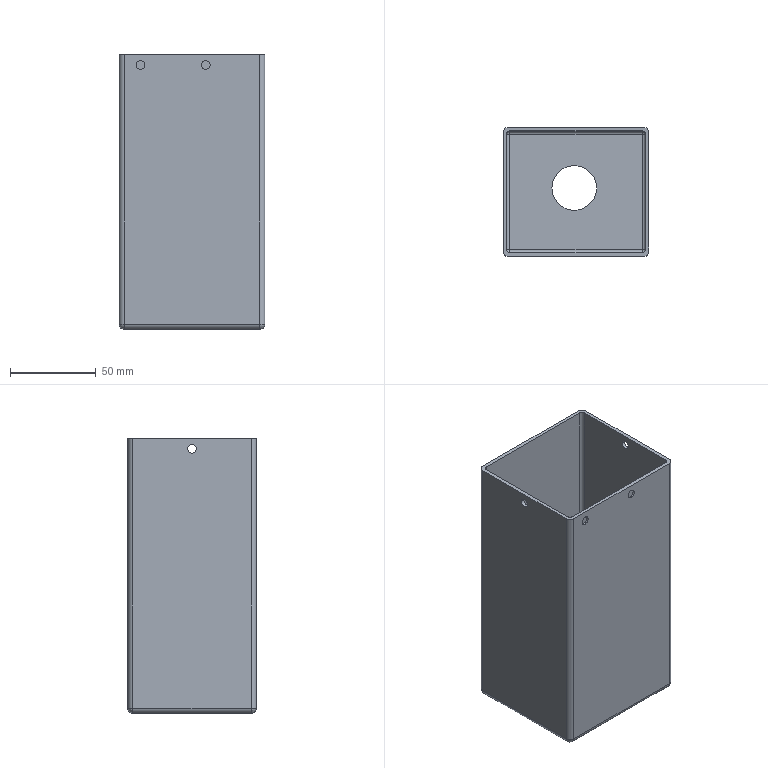Part | STEP file | Rotor step cover | 1 solid | 53 faces | box 85 x 75 x 160 mm | volume 109085 mm3 | cylinder 30 | plane 15 | spline 8 | commonest cylinder face diameters 5 x12 4 x8 6 x8 26 x2